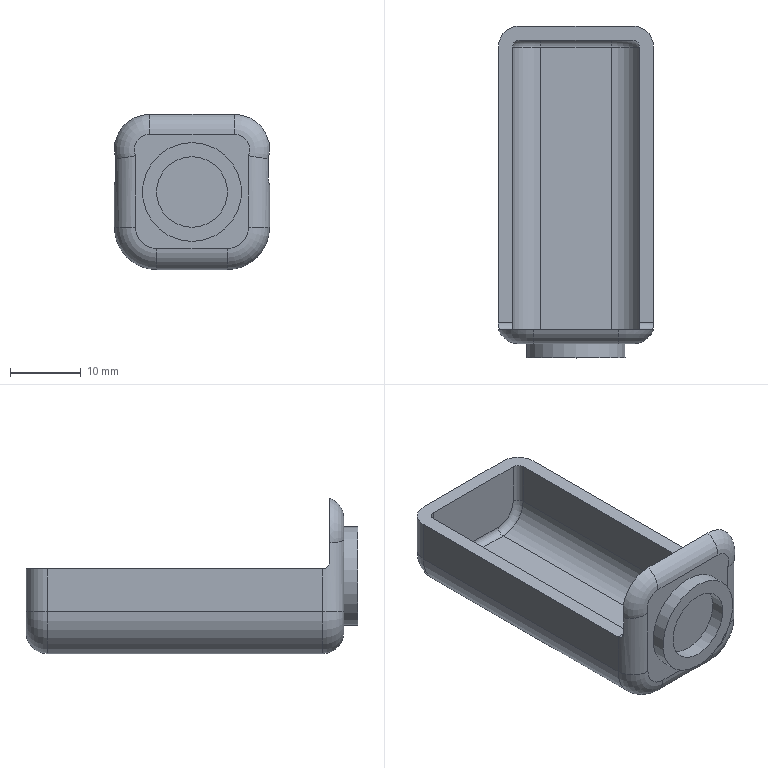Part | NX | features BLEND 5, DATUM_CSYS 4, SKETCH 3, EXTRUDE 2, SHELL 1, SWP104 1 | 1 solid | 39 faces | box 22 x 47 x 22 mm | volume 4457 mm3 | cylinder 18 | plane 13 | torus 8 | commonest cylinder face diameters 6 x7 2 x5 8 x2 12 x2 10 x1 14 x1
STEP:
#1=CARTESIAN_POINT('',(10.828,4.,2.));
#2=VERTEX_POINT('',#1);
#3=CARTESIAN_POINT('',(9.,4.,2.));
#4=VERTEX_POINT('',#3);
#5=CARTESIAN_POINT('',(-11.,4.,2.));
#6=DIRECTION('',(-1.,0.,0.));
#7=VECTOR('',#6,1000.);
#8=LINE('',#5,#7);
#9=EDGE_CURVE('',#2,#4,#8,.T.);
#10=ORIENTED_EDGE('',*,*,#9,.F.);
#11=CARTESIAN_POINT('',(11.,5.,1.));
#12=VERTEX_POINT('',#11);
#13=CARTESIAN_POINT('',(10.828,4.,2.));
#14=CARTESIAN_POINT('',(10.828,4.,1.468));
#15=CARTESIAN_POINT('',(11.,4.468,1.));
#16=CARTESIAN_POINT('',(11.,5.,1.));
#17=B_SPLINE_CURVE_WITH_KNOTS('',3,(#13,#14,#15,#16),.UNSPECIFIED.,.F.,.F.,(4,4),(0.,0.001574),.UNSPECIFIED.);
#18=EDGE_CURVE('',#2,#12,#17,.T.);
#19=ORIENTED_EDGE('',*,*,#18,.T.);
#20=CARTESIAN_POINT('',(9.,5.,1.));
#21=VERTEX_POINT('',#20);
#22=CARTESIAN_POINT('',(11.,5.,1.));
#23=DIRECTION('',(-1.,0.,0.));
#24=VECTOR('',#23,1000.);
#25=LINE('',#22,#24);
#26=EDGE_CURVE('',#21,#12,#25,.F.);
#27=ORIENTED_EDGE('',*,*,#26,.F.);
#28=CARTESIAN_POINT('',(9.,5.,2.));
#29=DIRECTION('',(-1.,0.,0.));
#30=DIRECTION('',(0.,0.,1.));
#31=AXIS2_PLACEMENT_3D('',#28,#29,#30);
#32=CIRCLE('',#31,1.);
#33=EDGE_CURVE('',#21,#4,#32,.T.);
#34=ORIENTED_EDGE('',*,*,#33,.T.);
#35=EDGE_LOOP('',(#10,#19,#27,#34));
#36=FACE_BOUND('',#35,.T.);
#37=CARTESIAN_POINT('',(-56.,5.,2.));
#38=DIRECTION('',(1.,0.,0.));
#39=DIRECTION('',(0.,0.,-1.));
#40=AXIS2_PLACEMENT_3D('',#37,#38,#39);
#41=CYLINDRICAL_SURFACE('',#40,1.);
#42=ADVANCED_FACE('',(#36),#41,.F.);
#43=CARTESIAN_POINT('',(-8.,47.,1.));
#44=VERTEX_POINT('',#43);
#45=CARTESIAN_POINT('',(8.,47.,1.));
#46=VERTEX_POINT('',#45);
#47=CARTESIAN_POINT('',(0.,47.,1.));
#48=DIRECTION('',(1.,0.,0.));
#49=VECTOR('',#48,1000.);
#50=LINE('',#47,#49);
#51=EDGE_CURVE('',#44,#46,#50,.T.);
#52=ORIENTED_EDGE('',*,*,#51,.T.);
#53=CARTESIAN_POINT('',(8.,47.,-5.));
#54=VERTEX_POINT('',#53);
#55=CARTESIAN_POINT('',(8.,47.,-5.));
#56=DIRECTION('',(0.,0.,-1.));
#57=VECTOR('',#56,1000.);
#58=LINE('',#55,#57);
#59=EDGE_CURVE('',#46,#54,#58,.T.);
#60=ORIENTED_EDGE('',*,*,#59,.T.);
#61=CARTESIAN_POINT('',(5.,47.,-8.));
#62=VERTEX_POINT('',#61);
#63=CARTESIAN_POINT('',(5.,47.,-5.));
#64=DIRECTION('',(0.,1.,0.));
#65=DIRECTION('',(0.,0.,1.));
#66=AXIS2_PLACEMENT_3D('',#63,#64,#65);
#67=CIRCLE('',#66,3.);
#68=EDGE_CURVE('',#54,#62,#67,.T.);
#69=ORIENTED_EDGE('',*,*,#68,.T.);
#70=CARTESIAN_POINT('',(-5.,47.,-8.));
#71=VERTEX_POINT('',#70);
#72=CARTESIAN_POINT('',(-5.,47.,-8.));
#73=DIRECTION('',(-1.,0.,0.));
#74=VECTOR('',#73,1000.);
#75=LINE('',#72,#74);
#76=EDGE_CURVE('',#62,#71,#75,.T.);
#77=ORIENTED_EDGE('',*,*,#76,.T.);
#78=CARTESIAN_POINT('',(-8.,47.,-5.));
#79=VERTEX_POINT('',#78);
#80=CARTESIAN_POINT('',(-5.,47.,-5.));
#81=DIRECTION('',(0.,1.,0.));
#82=DIRECTION('',(0.,0.,1.));
#83=AXIS2_PLACEMENT_3D('',#80,#81,#82);
#84=CIRCLE('',#83,3.);
#85=EDGE_CURVE('',#71,#79,#84,.T.);
#86=ORIENTED_EDGE('',*,*,#85,.T.);
#87=CARTESIAN_POINT('',(-8.,47.,1.));
#88=DIRECTION('',(0.,0.,1.));
#89=VECTOR('',#88,1000.);
#90=LINE('',#87,#89);
#91=EDGE_CURVE('',#79,#44,#90,.T.);
#92=ORIENTED_EDGE('',*,*,#91,.T.);
#93=EDGE_LOOP('',(#52,#60,#69,#77,#86,#92));
#94=FACE_BOUND('',#93,.T.);
#95=CARTESIAN_POINT('',(0.,47.,0.));
#96=DIRECTION('',(0.,1.,0.));
#97=DIRECTION('',(0.,0.,1.));
#98=AXIS2_PLACEMENT_3D('',#95,#96,#97);
#99=PLANE('',#98);
#100=ADVANCED_FACE('',(#94),#99,.T.);
#101=CARTESIAN_POINT('',(11.,44.,1.));
#102=VERTEX_POINT('',#101);
#103=CARTESIAN_POINT('',(11.,47.,1.));
#104=DIRECTION('',(0.,1.,0.));
#105=VECTOR('',#104,1000.);
#106=LINE('',#103,#105);
#107=EDGE_CURVE('',#12,#102,#106,.T.);
#108=ORIENTED_EDGE('',*,*,#107,.F.);
#109=CARTESIAN_POINT('',(11.,5.,-5.));
#110=VERTEX_POINT('',#109);
#111=CARTESIAN_POINT('',(11.,5.,11.));
#112=DIRECTION('',(0.,0.,-1.));
#113=VECTOR('',#112,1000.);
#114=LINE('',#111,#113);
#115=EDGE_CURVE('',#12,#110,#114,.T.);
#116=ORIENTED_EDGE('',*,*,#115,.T.);
#117=CARTESIAN_POINT('',(11.,44.,-5.));
#118=VERTEX_POINT('',#117);
#119=CARTESIAN_POINT('',(11.,47.,-5.));
#120=DIRECTION('',(0.,-1.,0.));
#121=VECTOR('',#120,1000.);
#122=LINE('',#119,#121);
#123=EDGE_CURVE('',#110,#118,#122,.F.);
#124=ORIENTED_EDGE('',*,*,#123,.T.);
#125=CARTESIAN_POINT('',(11.,44.,1.));
#126=DIRECTION('',(0.,0.,-1.));
#127=VECTOR('',#126,1000.);
#128=LINE('',#125,#127);
#129=EDGE_CURVE('',#118,#102,#128,.F.);
#130=ORIENTED_EDGE('',*,*,#129,.T.);
#131=EDGE_LOOP('',(#108,#116,#124,#130));
#132=FACE_BOUND('',#131,.T.);
#133=CARTESIAN_POINT('',(11.,47.,11.));
#134=DIRECTION('',(-1.,0.,0.));
#135=DIRECTION('',(0.,0.,1.));
#136=AXIS2_PLACEMENT_3D('',#133,#134,#135);
#137=PLANE('',#136);
#138=ADVANCED_FACE('',(#132),#137,.F.);
#139=CARTESIAN_POINT('',(-11.,44.,-5.));
#140=VERTEX_POINT('',#139);
#141=CARTESIAN_POINT('',(-11.,5.,-5.));
#142=VERTEX_POINT('',#141);
#143=CARTESIAN_POINT('',(-11.,47.,-5.));
#144=DIRECTION('',(0.,-1.,0.));
#145=VECTOR('',#144,1000.);
#146=LINE('',#143,#145);
#147=EDGE_CURVE('',#140,#142,#146,.T.);
#148=ORIENTED_EDGE('',*,*,#147,.T.);
#149=CARTESIAN_POINT('',(-11.,5.,1.));
#150=VERTEX_POINT('',#149);
#151=CARTESIAN_POINT('',(-11.,5.,-11.));
#152=DIRECTION('',(0.,0.,1.));
#153=VECTOR('',#152,1000.);
#154=LINE('',#151,#153);
#155=EDGE_CURVE('',#142,#150,#154,.T.);
#156=ORIENTED_EDGE('',*,*,#155,.T.);
#157=CARTESIAN_POINT('',(-11.,44.,1.));
#158=VERTEX_POINT('',#157);
#159=CARTESIAN_POINT('',(-11.,47.,1.));
#160=DIRECTION('',(0.,-1.,0.));
#161=VECTOR('',#160,1000.);
#162=LINE('',#159,#161);
#163=EDGE_CURVE('',#158,#150,#162,.T.);
#164=ORIENTED_EDGE('',*,*,#163,.F.);
#165=CARTESIAN_POINT('',(-11.,44.,-5.));
#166=DIRECTION('',(0.,0.,1.));
#167=VECTOR('',#166,1000.);
#168=LINE('',#165,#167);
#169=EDGE_CURVE('',#158,#140,#168,.F.);
#170=ORIENTED_EDGE('',*,*,#169,.T.);
#171=EDGE_LOOP('',(#148,#156,#164,#170));
#172=FACE_BOUND('',#171,.T.);
#173=CARTESIAN_POINT('',(-11.,47.,-11.));
#174=DIRECTION('',(1.,0.,0.));
#175=DIRECTION('',(0.,0.,-1.));
#176=AXIS2_PLACEMENT_3D('',#173,#174,#175);
#177=PLANE('',#176);
#178=ADVANCED_FACE('',(#172),#177,.F.);
#179=CARTESIAN_POINT('',(0.,0.,5.));
#180=VERTEX_POINT('',#179);
#181=CARTESIAN_POINT('',(0.,0.,0.));
#182=DIRECTION('',(0.,1.,0.));
#183=DIRECTION('',(0.,0.,1.));
#184=AXIS2_PLACEMENT_3D('',#181,#182,#183);
#185=CIRCLE('',#184,5.);
#186=EDGE_CURVE('',#180,#180,#185,.T.);
#187=ORIENTED_EDGE('',*,*,#186,.F.);
#188=EDGE_LOOP('',(#187));
#189=FACE_BOUND('',#188,.T.);
#190=CARTESIAN_POINT('',(0.,2.,5.));
#191=VERTEX_POINT('',#190);
#192=CARTESIAN_POINT('',(0.,2.,0.));
#193=DIRECTION('',(0.,1.,0.));
#194=DIRECTION('',(0.,0.,1.));
#195=AXIS2_PLACEMENT_3D('',#192,#193,#194);
#196=CIRCLE('',#195,5.);
#197=EDGE_CURVE('',#191,#191,#196,.T.);
#198=ORIENTED_EDGE('',*,*,#197,.T.);
#199=EDGE_LOOP('',(#198));
#200=FACE_BOUND('',#199,.T.);
#201=CARTESIAN_POINT('',(0.,0.,0.));
#202=DIRECTION('',(0.,1.,0.));
#203=DIRECTION('',(0.,0.,1.));
#204=AXIS2_PLACEMENT_3D('',#201,#202,#203);
#205=CYLINDRICAL_SURFACE('',#204,5.);
#206=ADVANCED_FACE('',(#189,#200),#205,.F.);
#207=CARTESIAN_POINT('',(0.,0.,7.));
#208=VERTEX_POINT('',#207);
#209=CARTESIAN_POINT('',(0.,0.,0.));
#210=DIRECTION('',(0.,1.,0.));
#211=DIRECTION('',(0.,0.,1.));
#212=AXIS2_PLACEMENT_3D('',#209,#210,#211);
#213=CIRCLE('',#212,7.);
#214=EDGE_CURVE('',#208,#208,#213,.T.);
#215=ORIENTED_EDGE('',*,*,#214,.F.);
#216=EDGE_LOOP('',(#215));
#217=FACE_BOUND('',#216,.T.);
#218=ORIENTED_EDGE('',*,*,#186,.T.);
#219=EDGE_LOOP('',(#218));
#220=FACE_BOUND('',#219,.T.);
#221=CARTESIAN_POINT('',(5.,0.,0.));
#222=DIRECTION('',(0.,1.,0.));
#223=DIRECTION('',(0.,0.,1.));
#224=AXIS2_PLACEMENT_3D('',#221,#222,#223);
#225=PLANE('',#224);
#226=ADVANCED_FACE('',(#217,#220),#225,.F.);
#227=CARTESIAN_POINT('',(0.,2.,7.));
#228=VERTEX_POINT('',#227);
#229=CARTESIAN_POINT('',(0.,2.,0.));
#230=DIRECTION('',(0.,1.,0.));
#231=DIRECTION('',(0.,0.,1.));
#232=AXIS2_PLACEMENT_3D('',#229,#230,#231);
#233=CIRCLE('',#232,7.);
#234=EDGE_CURVE('',#228,#228,#233,.T.);
#235=ORIENTED_EDGE('',*,*,#234,.F.);
#236=EDGE_LOOP('',(#235));
#237=FACE_BOUND('',#236,.T.);
#238=ORIENTED_EDGE('',*,*,#214,.T.);
#239=EDGE_LOOP('',(#238));
#240=FACE_BOUND('',#239,.T.);
#241=CARTESIAN_POINT('',(0.,0.,0.));
#242=DIRECTION('',(0.,1.,0.));
#243=DIRECTION('',(0.,0.,1.));
#244=AXIS2_PLACEMENT_3D('',#241,#242,#243);
#245=CYLINDRICAL_SURFACE('',#244,7.);
#246=ADVANCED_FACE('',(#237,#240),#245,.T.);
#247=CARTESIAN_POINT('',(-8.,2.,-5.));
#248=VERTEX_POINT('',#247);
#249=CARTESIAN_POINT('',(-5.,2.,-8.));
#250=VERTEX_POINT('',#249);
#251=CARTESIAN_POINT('',(-5.,2.,-5.));
#252=DIRECTION('',(0.,1.,0.));
#253=DIRECTION('',(0.,0.,1.));
#254=AXIS2_PLACEMENT_3D('',#251,#252,#253);
#255=CIRCLE('',#254,3.);
#256=EDGE_CURVE('',#248,#250,#255,.F.);
#257=ORIENTED_EDGE('',*,*,#256,.T.);
#258=CARTESIAN_POINT('',(5.,2.,-8.));
#259=VERTEX_POINT('',#258);
#260=CARTESIAN_POINT('',(0.,2.,-8.));
#261=DIRECTION('',(-1.,0.,0.));
#262=VECTOR('',#261,1000.);
#263=LINE('',#260,#262);
#264=EDGE_CURVE('',#250,#259,#263,.F.);
#265=ORIENTED_EDGE('',*,*,#264,.T.);
#266=CARTESIAN_POINT('',(8.,2.,-5.));
#267=VERTEX_POINT('',#266);
#268=CARTESIAN_POINT('',(5.,2.,-5.));
#269=DIRECTION('',(0.,1.,0.));
#270=DIRECTION('',(0.,0.,1.));
#271=AXIS2_PLACEMENT_3D('',#268,#269,#270);
#272=CIRCLE('',#271,3.);
#273=EDGE_CURVE('',#259,#267,#272,.F.);
#274=ORIENTED_EDGE('',*,*,#273,.T.);
#275=CARTESIAN_POINT('',(8.,2.,5.154));
#276=VERTEX_POINT('',#275);
#277=CARTESIAN_POINT('',(8.,2.,0.));
#278=DIRECTION('',(0.,0.,-1.));
#279=VECTOR('',#278,1000.);
#280=LINE('',#277,#279);
#281=EDGE_CURVE('',#267,#276,#280,.F.);
#282=ORIENTED_EDGE('',*,*,#281,.T.);
#283=CARTESIAN_POINT('',(6.,2.,8.172));
#284=VERTEX_POINT('',#283);
#285=CARTESIAN_POINT('',(6.,2.,6.));
#286=DIRECTION('',(0.,1.,0.));
#287=DIRECTION('',(0.,0.,1.));
#288=AXIS2_PLACEMENT_3D('',#285,#286,#287);
#289=CIRCLE('',#288,2.172);
#290=EDGE_CURVE('',#276,#284,#289,.F.);
#291=ORIENTED_EDGE('',*,*,#290,.T.);
#292=CARTESIAN_POINT('',(-6.,2.,8.172));
#293=VERTEX_POINT('',#292);
#294=CARTESIAN_POINT('',(0.,2.,8.172));
#295=DIRECTION('',(1.,0.,0.));
#296=VECTOR('',#295,1000.);
#297=LINE('',#294,#296);
#298=EDGE_CURVE('',#284,#293,#297,.F.);
#299=ORIENTED_EDGE('',*,*,#298,.T.);
#300=CARTESIAN_POINT('',(-8.,2.,5.154));
#301=VERTEX_POINT('',#300);
#302=CARTESIAN_POINT('',(-6.,2.,6.));
#303=DIRECTION('',(0.,1.,0.));
#304=DIRECTION('',(0.,0.,1.));
#305=AXIS2_PLACEMENT_3D('',#302,#303,#304);
#306=CIRCLE('',#305,2.172);
#307=EDGE_CURVE('',#293,#301,#306,.F.);
#308=ORIENTED_EDGE('',*,*,#307,.T.);
#309=CARTESIAN_POINT('',(-8.,2.,0.));
#310=DIRECTION('',(0.,0.,1.));
#311=VECTOR('',#310,1000.);
#312=LINE('',#309,#311);
#313=EDGE_CURVE('',#301,#248,#312,.F.);
#314=ORIENTED_EDGE('',*,*,#313,.T.);
#315=EDGE_LOOP('',(#257,#265,#274,#282,#291,#299,#308,#314));
#316=FACE_BOUND('',#315,.T.);
#317=ORIENTED_EDGE('',*,*,#234,.T.);
#318=EDGE_LOOP('',(#317));
#319=FACE_BOUND('',#318,.T.);
#320=CARTESIAN_POINT('',(0.,2.,0.));
#321=DIRECTION('',(0.,1.,0.));
#322=DIRECTION('',(0.,0.,1.));
#323=AXIS2_PLACEMENT_3D('',#320,#321,#322);
#324=PLANE('',#323);
#325=ADVANCED_FACE('',(#316,#319),#324,.F.);
#326=CARTESIAN_POINT('',(5.,44.,-11.));
#327=VERTEX_POINT('',#326);
#328=CARTESIAN_POINT('',(5.,5.,-11.));
#329=VERTEX_POINT('',#328);
#330=CARTESIAN_POINT('',(5.,47.,-11.));
#331=DIRECTION('',(0.,-1.,0.));
#332=VECTOR('',#331,1000.);
#333=LINE('',#330,#332);
#334=EDGE_CURVE('',#327,#329,#333,.T.);
#335=ORIENTED_EDGE('',*,*,#334,.T.);
#336=CARTESIAN_POINT('',(-5.,5.,-11.));
#337=VERTEX_POINT('',#336);
#338=CARTESIAN_POINT('',(11.,5.,-11.));
#339=DIRECTION('',(-1.,0.,0.));
#340=VECTOR('',#339,1000.);
#341=LINE('',#338,#340);
#342=EDGE_CURVE('',#329,#337,#341,.T.);
#343=ORIENTED_EDGE('',*,*,#342,.T.);
#344=CARTESIAN_POINT('',(-5.,44.,-11.));
#345=VERTEX_POINT('',#344);
#346=CARTESIAN_POINT('',(-5.,47.,-11.));
#347=DIRECTION('',(0.,-1.,0.));
#348=VECTOR('',#347,1000.);
#349=LINE('',#346,#348);
#350=EDGE_CURVE('',#337,#345,#349,.F.);
#351=ORIENTED_EDGE('',*,*,#350,.T.);
#352=CARTESIAN_POINT('',(5.,44.,-11.));
#353=DIRECTION('',(-1.,0.,0.));
#354=VECTOR('',#353,1000.);
#355=LINE('',#352,#354);
#356=EDGE_CURVE('',#345,#327,#355,.F.);
#357=ORIENTED_EDGE('',*,*,#356,.T.);
#358=EDGE_LOOP('',(#335,#343,#351,#357));
#359=FACE_BOUND('',#358,.T.);
#360=CARTESIAN_POINT('',(11.,47.,-11.));
#361=DIRECTION('',(0.,0.,1.));
#362=DIRECTION('',(1.,0.,0.));
#363=AXIS2_PLACEMENT_3D('',#360,#361,#362);
#364=PLANE('',#363);
#365=ADVANCED_FACE('',(#359),#364,.F.);
#366=ORIENTED_EDGE('',*,*,#197,.F.);
#367=EDGE_LOOP('',(#366));
#368=FACE_BOUND('',#367,.T.);
#369=CARTESIAN_POINT('',(0.,2.,0.));
#370=DIRECTION('',(0.,1.,0.));
#371=DIRECTION('',(0.,0.,1.));
#372=AXIS2_PLACEMENT_3D('',#369,#370,#371);
#373=PLANE('',#372);
#374=ADVANCED_FACE('',(#368),#373,.F.);
#375=CARTESIAN_POINT('',(-6.,4.,11.));
#376=VERTEX_POINT('',#375);
#377=CARTESIAN_POINT('',(6.,4.,11.));
#378=VERTEX_POINT('',#377);
#379=CARTESIAN_POINT('',(-56.,4.,11.));
#380=DIRECTION('',(1.,0.,0.));
#381=VECTOR('',#380,1000.);
#382=LINE('',#379,#381);
#383=EDGE_CURVE('',#376,#378,#382,.T.);
#384=ORIENTED_EDGE('',*,*,#383,.T.);
#385=CARTESIAN_POINT('',(10.828,4.,4.701));
#386=VERTEX_POINT('',#385);
#387=CARTESIAN_POINT('',(6.,4.,6.));
#388=DIRECTION('',(0.,1.,0.));
#389=DIRECTION('',(0.,0.,1.));
#390=AXIS2_PLACEMENT_3D('',#387,#388,#389);
#391=CIRCLE('',#390,5.);
#392=EDGE_CURVE('',#378,#386,#391,.T.);
#393=ORIENTED_EDGE('',*,*,#392,.T.);
#394=CARTESIAN_POINT('',(10.828,4.,4.701));
#395=DIRECTION('',(0.,0.,-1.));
#396=VECTOR('',#395,1000.);
#397=LINE('',#394,#396);
#398=EDGE_CURVE('',#386,#2,#397,.T.);
#399=ORIENTED_EDGE('',*,*,#398,.T.);
#400=ORIENTED_EDGE('',*,*,#9,.T.);
#401=CARTESIAN_POINT('',(9.,4.,-5.));
#402=VERTEX_POINT('',#401);
#403=CARTESIAN_POINT('',(9.,4.,11.));
#404=DIRECTION('',(0.,0.,-1.));
#405=VECTOR('',#404,1000.);
#406=LINE('',#403,#405);
#407=EDGE_CURVE('',#4,#402,#406,.T.);
#408=ORIENTED_EDGE('',*,*,#407,.T.);
#409=CARTESIAN_POINT('',(5.,4.,-9.));
#410=VERTEX_POINT('',#409);
#411=CARTESIAN_POINT('',(5.,4.,-5.));
#412=DIRECTION('',(0.,1.,0.));
#413=DIRECTION('',(0.,0.,1.));
#414=AXIS2_PLACEMENT_3D('',#411,#412,#413);
#415=CIRCLE('',#414,4.);
#416=EDGE_CURVE('',#410,#402,#415,.F.);
#417=ORIENTED_EDGE('',*,*,#416,.F.);
#418=CARTESIAN_POINT('',(-5.,4.,-9.));
#419=VERTEX_POINT('',#418);
#420=CARTESIAN_POINT('',(11.,4.,-9.));
#421=DIRECTION('',(-1.,0.,0.));
#422=VECTOR('',#421,1000.);
#423=LINE('',#420,#422);
#424=EDGE_CURVE('',#410,#419,#423,.T.);
#425=ORIENTED_EDGE('',*,*,#424,.T.);
#426=CARTESIAN_POINT('',(-9.,4.,-5.));
#427=VERTEX_POINT('',#426);
#428=CARTESIAN_POINT('',(-5.,4.,-5.));
#429=DIRECTION('',(0.,1.,0.));
#430=DIRECTION('',(0.,0.,1.));
#431=AXIS2_PLACEMENT_3D('',#428,#429,#430);
#432=CIRCLE('',#431,4.);
#433=EDGE_CURVE('',#427,#419,#432,.F.);
#434=ORIENTED_EDGE('',*,*,#433,.F.);
#435=CARTESIAN_POINT('',(-9.,4.,2.));
#436=VERTEX_POINT('',#435);
#437=CARTESIAN_POINT('',(-9.,4.,-11.));
#438=DIRECTION('',(0.,0.,1.));
#439=VECTOR('',#438,1000.);
#440=LINE('',#437,#439);
#441=EDGE_CURVE('',#427,#436,#440,.T.);
#442=ORIENTED_EDGE('',*,*,#441,.T.);
#443=CARTESIAN_POINT('',(-10.828,4.,2.));
#444=VERTEX_POINT('',#443);
#445=CARTESIAN_POINT('',(-11.,4.,2.));
#446=DIRECTION('',(-1.,0.,0.));
#447=VECTOR('',#446,1000.);
#448=LINE('',#445,#447);
#449=EDGE_CURVE('',#436,#444,#448,.T.);
#450=ORIENTED_EDGE('',*,*,#449,.T.);
#451=CARTESIAN_POINT('',(-10.828,4.,4.701));
#452=VERTEX_POINT('',#451);
#453=CARTESIAN_POINT('',(-10.828,4.,2.));
#454=DIRECTION('',(0.,0.,1.));
#455=VECTOR('',#454,1000.);
#456=LINE('',#453,#455);
#457=EDGE_CURVE('',#444,#452,#456,.T.);
#458=ORIENTED_EDGE('',*,*,#457,.T.);
#459=CARTESIAN_POINT('',(-6.,4.,6.));
#460=DIRECTION('',(0.,1.,0.));
#461=DIRECTION('',(0.,0.,1.));
#462=AXIS2_PLACEMENT_3D('',#459,#460,#461);
#463=CIRCLE('',#462,5.);
#464=EDGE_CURVE('',#452,#376,#463,.T.);
#465=ORIENTED_EDGE('',*,*,#464,.T.);
#466=EDGE_LOOP('',(#384,#393,#399,#400,#408,#417,#425,#434,#442,#450,#458,#465));
#467=FACE_BOUND('',#466,.T.);
#468=CARTESIAN_POINT('',(-56.,4.,1.));
#469=DIRECTION('',(0.,1.,0.));
#470=DIRECTION('',(0.,0.,1.));
#471=AXIS2_PLACEMENT_3D('',#468,#469,#470);
#472=PLANE('',#471);
#473=ADVANCED_FACE('',(#467),#472,.T.);
#474=CARTESIAN_POINT('',(9.,44.,1.));
#475=VERTEX_POINT('',#474);
#476=CARTESIAN_POINT('',(9.,47.,1.));
#477=DIRECTION('',(0.,1.,0.));
#478=VECTOR('',#477,1000.);
#479=LINE('',#476,#478);
#480=EDGE_CURVE('',#21,#475,#479,.T.);
#481=ORIENTED_EDGE('',*,*,#480,.F.);
#482=ORIENTED_EDGE('',*,*,#26,.T.);
#483=ORIENTED_EDGE('',*,*,#107,.T.);
#484=CARTESIAN_POINT('',(8.,44.,1.));
#485=DIRECTION('',(0.,0.,1.));
#486=DIRECTION('',(1.,0.,0.));
#487=AXIS2_PLACEMENT_3D('',#484,#485,#486);
#488=CIRCLE('',#487,3.);
#489=EDGE_CURVE('',#102,#46,#488,.T.);
#490=ORIENTED_EDGE('',*,*,#489,.T.);
#491=ORIENTED_EDGE('',*,*,#51,.F.);
#492=CARTESIAN_POINT('',(-8.,44.,1.));
#493=DIRECTION('',(0.,0.,1.));
#494=DIRECTION('',(1.,0.,0.));
#495=AXIS2_PLACEMENT_3D('',#492,#493,#494);
#496=CIRCLE('',#495,3.);
#497=EDGE_CURVE('',#44,#158,#496,.T.);
#498=ORIENTED_EDGE('',*,*,#497,.T.);
#499=ORIENTED_EDGE('',*,*,#163,.T.);
#500=CARTESIAN_POINT('',(-9.,5.,1.));
#501=VERTEX_POINT('',#500);
#502=CARTESIAN_POINT('',(11.,5.,1.));
#503=DIRECTION('',(-1.,0.,0.));
#504=VECTOR('',#503,1000.);
#505=LINE('',#502,#504);
#506=EDGE_CURVE('',#150,#501,#505,.F.);
#507=ORIENTED_EDGE('',*,*,#506,.T.);
#508=CARTESIAN_POINT('',(-9.,44.,1.));
#509=VERTEX_POINT('',#508);
#510=CARTESIAN_POINT('',(-9.,47.,1.));
#511=DIRECTION('',(0.,-1.,0.));
#512=VECTOR('',#511,1000.);
#513=LINE('',#510,#512);
#514=EDGE_CURVE('',#509,#501,#513,.T.);
#515=ORIENTED_EDGE('',*,*,#514,.F.);
#516=CARTESIAN_POINT('',(-8.,45.,1.));
#517=VERTEX_POINT('',#516);
#518=CARTESIAN_POINT('',(-8.,44.,1.));
#519=DIRECTION('',(0.,0.,1.));
#520=DIRECTION('',(1.,0.,0.));
#521=AXIS2_PLACEMENT_3D('',#518,#519,#520);
#522=CIRCLE('',#521,1.);
#523=EDGE_CURVE('',#517,#509,#522,.T.);
#524=ORIENTED_EDGE('',*,*,#523,.F.);
#525=CARTESIAN_POINT('',(8.,45.,1.));
#526=VERTEX_POINT('',#525);
#527=CARTESIAN_POINT('',(0.,45.,1.));
#528=DIRECTION('',(1.,0.,0.));
#529=VECTOR('',#528,1000.);
#530=LINE('',#527,#529);
#531=EDGE_CURVE('',#517,#526,#530,.T.);
#532=ORIENTED_EDGE('',*,*,#531,.T.);
#533=CARTESIAN_POINT('',(8.,44.,1.));
#534=DIRECTION('',(0.,0.,1.));
#535=DIRECTION('',(1.,0.,0.));
#536=AXIS2_PLACEMENT_3D('',#533,#534,#535);
#537=CIRCLE('',#536,1.);
#538=EDGE_CURVE('',#475,#526,#537,.T.);
#539=ORIENTED_EDGE('',*,*,#538,.F.);
#540=EDGE_LOOP('',(#481,#482,#483,#490,#491,#498,#499,#507,#515,#524,#532,#539));
#541=FACE_BOUND('',#540,.T.);
#542=CARTESIAN_POINT('',(-56.,54.5,1.));
#543=DIRECTION('',(0.,0.,1.));
#544=DIRECTION('',(1.,0.,0.));
#545=AXIS2_PLACEMENT_3D('',#542,#543,#544);
#546=PLANE('',#545);
#547=ADVANCED_FACE('',(#541),#546,.T.);
#548=ORIENTED_EDGE('',*,*,#350,.F.);
#549=CARTESIAN_POINT('',(-5.,5.,-5.));
#550=DIRECTION('',(0.,1.,0.));
#551=DIRECTION('',(0.,0.,1.));
#552=AXIS2_PLACEMENT_3D('',#549,#550,#551);
#553=CIRCLE('',#552,6.);
#554=EDGE_CURVE('',#337,#142,#553,.T.);
#555=ORIENTED_EDGE('',*,*,#554,.T.);
#556=ORIENTED_EDGE('',*,*,#147,.F.);
#557=CARTESIAN_POINT('',(-5.,44.,-5.));
#558=DIRECTION('',(0.,1.,0.));
#559=DIRECTION('',(0.,0.,1.));
#560=AXIS2_PLACEMENT_3D('',#557,#558,#559);
#561=CIRCLE('',#560,6.);
#562=EDGE_CURVE('',#140,#345,#561,.F.);
#563=ORIENTED_EDGE('',*,*,#562,.T.);
#564=EDGE_LOOP('',(#548,#555,#556,#563));
#565=FACE_BOUND('',#564,.T.);
#566=CARTESIAN_POINT('',(-5.,47.,-5.));
#567=DIRECTION('',(0.,-1.,0.));
#568=DIRECTION('',(0.,0.,-1.));
#569=AXIS2_PLACEMENT_3D('',#566,#567,#568);
#570=CYLINDRICAL_SURFACE('',#569,6.);
#571=ADVANCED_FACE('',(#565),#570,.T.);
#572=ORIENTED_EDGE('',*,*,#123,.F.);
#573=CARTESIAN_POINT('',(5.,5.,-5.));
#574=DIRECTION('',(0.,1.,0.));
#575=DIRECTION('',(0.,0.,1.));
#576=AXIS2_PLACEMENT_3D('',#573,#574,#575);
#577=CIRCLE('',#576,6.);
#578=EDGE_CURVE('',#110,#329,#577,.T.);
#579=ORIENTED_EDGE('',*,*,#578,.T.);
#580=ORIENTED_EDGE('',*,*,#334,.F.);
#581=CARTESIAN_POINT('',(5.,44.,-5.));
#582=DIRECTION('',(0.,1.,0.));
#583=DIRECTION('',(0.,0.,1.));
#584=AXIS2_PLACEMENT_3D('',#581,#582,#583);
#585=CIRCLE('',#584,6.);
#586=EDGE_CURVE('',#327,#118,#585,.F.);
#587=ORIENTED_EDGE('',*,*,#586,.T.);
#588=EDGE_LOOP('',(#572,#579,#580,#587));
#589=FACE_BOUND('',#588,.T.);
#590=CARTESIAN_POINT('',(5.,47.,-5.));
#591=DIRECTION('',(0.,-1.,0.));
#592=DIRECTION('',(0.,0.,-1.));
#593=AXIS2_PLACEMENT_3D('',#590,#591,#592);
#594=CYLINDRICAL_SURFACE('',#593,6.);
#595=ADVANCED_FACE('',(#589),#594,.T.);
#596=ORIENTED_EDGE('',*,*,#506,.F.);
#597=CARTESIAN_POINT('',(-11.,5.,1.));
#598=CARTESIAN_POINT('',(-11.,4.468,1.));
#599=CARTESIAN_POINT('',(-10.828,4.,1.468));
#600=CARTESIAN_POINT('',(-10.828,4.,2.));
#601=B_SPLINE_CURVE_WITH_KNOTS('',3,(#597,#598,#599,#600),.UNSPECIFIED.,.F.,.F.,(4,4),(0.,0.001574),.UNSPECIFIED.);
#602=EDGE_CURVE('',#150,#444,#601,.T.);
#603=ORIENTED_EDGE('',*,*,#602,.T.);
#604=ORIENTED_EDGE('',*,*,#449,.F.);
#605=CARTESIAN_POINT('',(-9.,5.,2.));
#606=DIRECTION('',(1.,0.,0.));
#607=DIRECTION('',(0.,0.,-1.));
#608=AXIS2_PLACEMENT_3D('',#605,#606,#607);
#609=CIRCLE('',#608,1.);
#610=EDGE_CURVE('',#436,#501,#609,.T.);
#611=ORIENTED_EDGE('',*,*,#610,.T.);
#612=EDGE_LOOP('',(#596,#603,#604,#611));
#613=FACE_BOUND('',#612,.T.);
#614=CARTESIAN_POINT('',(-56.,5.,2.));
#615=DIRECTION('',(1.,0.,0.));
#616=DIRECTION('',(0.,0.,-1.));
#617=AXIS2_PLACEMENT_3D('',#614,#615,#616);
#618=CYLINDRICAL_SURFACE('',#617,1.);
#619=ADVANCED_FACE('',(#613),#618,.F.);
#620=ORIENTED_EDGE('',*,*,#497,.F.);
#621=ORIENTED_EDGE('',*,*,#91,.F.);
#622=CARTESIAN_POINT('',(-8.,44.,-5.));
#623=DIRECTION('',(0.,0.,-1.));
#624=DIRECTION('',(-1.,0.,0.));
#625=AXIS2_PLACEMENT_3D('',#622,#623,#624);
#626=CIRCLE('',#625,3.);
#627=EDGE_CURVE('',#140,#79,#626,.T.);
#628=ORIENTED_EDGE('',*,*,#627,.F.);
#629=ORIENTED_EDGE('',*,*,#169,.F.);
#630=EDGE_LOOP('',(#620,#621,#628,#629));
#631=FACE_BOUND('',#630,.T.);
#632=CARTESIAN_POINT('',(-8.,44.,0.));
#633=DIRECTION('',(0.,0.,-1.));
#634=DIRECTION('',(-1.,0.,0.));
#635=AXIS2_PLACEMENT_3D('',#632,#633,#634);
#636=CYLINDRICAL_SURFACE('',#635,3.);
#637=ADVANCED_FACE('',(#631),#636,.T.);
#638=ORIENTED_EDGE('',*,*,#627,.T.);
#639=ORIENTED_EDGE('',*,*,#85,.F.);
#640=CARTESIAN_POINT('',(-5.,44.,-8.));
#641=DIRECTION('',(1.,0.,0.));
#642=DIRECTION('',(0.,0.,-1.));
#643=AXIS2_PLACEMENT_3D('',#640,#641,#642);
#644=CIRCLE('',#643,3.);
#645=EDGE_CURVE('',#345,#71,#644,.T.);
#646=ORIENTED_EDGE('',*,*,#645,.F.);
#647=ORIENTED_EDGE('',*,*,#562,.F.);
#648=EDGE_LOOP('',(#638,#639,#646,#647));
#649=FACE_BOUND('',#648,.T.);
#650=CARTESIAN_POINT('',(-5.,44.,-5.));
#651=DIRECTION('',(0.,1.,0.));
#652=DIRECTION('',(0.,0.,1.));
#653=AXIS2_PLACEMENT_3D('',#650,#651,#652);
#654=TOROIDAL_SURFACE('',#653,3.,3.);
#655=ADVANCED_FACE('',(#649),#654,.T.);
#656=ORIENTED_EDGE('',*,*,#645,.T.);
#657=ORIENTED_EDGE('',*,*,#76,.F.);
#658=CARTESIAN_POINT('',(5.,44.,-8.));
#659=DIRECTION('',(1.,0.,0.));
#660=DIRECTION('',(0.,0.,-1.));
#661=AXIS2_PLACEMENT_3D('',#658,#659,#660);
#662=CIRCLE('',#661,3.);
#663=EDGE_CURVE('',#327,#62,#662,.T.);
#664=ORIENTED_EDGE('',*,*,#663,.F.);
#665=ORIENTED_EDGE('',*,*,#356,.F.);
#666=EDGE_LOOP('',(#656,#657,#664,#665));
#667=FACE_BOUND('',#666,.T.);
#668=CARTESIAN_POINT('',(0.,44.,-8.));
#669=DIRECTION('',(1.,0.,0.));
#670=DIRECTION('',(0.,0.,-1.));
#671=AXIS2_PLACEMENT_3D('',#668,#669,#670);
#672=CYLINDRICAL_SURFACE('',#671,3.);
#673=ADVANCED_FACE('',(#667),#672,.T.);
#674=ORIENTED_EDGE('',*,*,#663,.T.);
#675=ORIENTED_EDGE('',*,*,#68,.F.);
#676=CARTESIAN_POINT('',(8.,44.,-5.));
#677=DIRECTION('',(0.,0.,1.));
#678=DIRECTION('',(1.,0.,0.));
#679=AXIS2_PLACEMENT_3D('',#676,#677,#678);
#680=CIRCLE('',#679,3.);
#681=EDGE_CURVE('',#118,#54,#680,.T.);
#682=ORIENTED_EDGE('',*,*,#681,.F.);
#683=ORIENTED_EDGE('',*,*,#586,.F.);
#684=EDGE_LOOP('',(#674,#675,#682,#683));
#685=FACE_BOUND('',#684,.T.);
#686=CARTESIAN_POINT('',(5.,44.,-5.));
#687=DIRECTION('',(0.,1.,0.));
#688=DIRECTION('',(0.,0.,1.));
#689=AXIS2_PLACEMENT_3D('',#686,#687,#688);
#690=TOROIDAL_SURFACE('',#689,3.,3.);
#691=ADVANCED_FACE('',(#685),#690,.T.);
#692=ORIENTED_EDGE('',*,*,#489,.F.);
#693=ORIENTED_EDGE('',*,*,#129,.F.);
#694=ORIENTED_EDGE('',*,*,#681,.T.);
#695=ORIENTED_EDGE('',*,*,#59,.F.);
#696=EDGE_LOOP('',(#692,#693,#694,#695));
#697=FACE_BOUND('',#696,.T.);
#698=CARTESIAN_POINT('',(8.,44.,0.));
#699=DIRECTION('',(0.,0.,1.));
#700=DIRECTION('',(1.,0.,0.));
#701=AXIS2_PLACEMENT_3D('',#698,#699,#700);
#702=CYLINDRICAL_SURFACE('',#701,3.);
#703=ADVANCED_FACE('',(#697),#702,.T.);
#704=ORIENTED_EDGE('',*,*,#531,.F.);
#705=CARTESIAN_POINT('',(-8.,45.,-5.));
#706=VERTEX_POINT('',#705);
#707=CARTESIAN_POINT('',(-8.,45.,0.));
#708=DIRECTION('',(0.,0.,1.));
#709=VECTOR('',#708,1000.);
#710=LINE('',#707,#709);
#711=EDGE_CURVE('',#706,#517,#710,.T.);
#712=ORIENTED_EDGE('',*,*,#711,.F.);
#713=CARTESIAN_POINT('',(-5.,45.,-8.));
#714=VERTEX_POINT('',#713);
#715=CARTESIAN_POINT('',(-5.,45.,-5.));
#716=DIRECTION('',(0.,1.,0.));
#717=DIRECTION('',(0.,0.,1.));
#718=AXIS2_PLACEMENT_3D('',#715,#716,#717);
#719=CIRCLE('',#718,3.);
#720=EDGE_CURVE('',#714,#706,#719,.T.);
#721=ORIENTED_EDGE('',*,*,#720,.F.);
#722=CARTESIAN_POINT('',(5.,45.,-8.));
#723=VERTEX_POINT('',#722);
#724=CARTESIAN_POINT('',(0.,45.,-8.));
#725=DIRECTION('',(1.,0.,0.));
#726=VECTOR('',#725,1000.);
#727=LINE('',#724,#726);
#728=EDGE_CURVE('',#723,#714,#727,.F.);
#729=ORIENTED_EDGE('',*,*,#728,.F.);
#730=CARTESIAN_POINT('',(8.,45.,-5.));
#731=VERTEX_POINT('',#730);
#732=CARTESIAN_POINT('',(5.,45.,-5.));
#733=DIRECTION('',(0.,1.,0.));
#734=DIRECTION('',(0.,0.,1.));
#735=AXIS2_PLACEMENT_3D('',#732,#733,#734);
#736=CIRCLE('',#735,3.);
#737=EDGE_CURVE('',#731,#723,#736,.T.);
#738=ORIENTED_EDGE('',*,*,#737,.F.);
#739=CARTESIAN_POINT('',(8.,45.,0.));
#740=DIRECTION('',(0.,0.,1.));
#741=VECTOR('',#740,1000.);
#742=LINE('',#739,#741);
#743=EDGE_CURVE('',#526,#731,#742,.F.);
#744=ORIENTED_EDGE('',*,*,#743,.F.);
#745=EDGE_LOOP('',(#704,#712,#721,#729,#738,#744));
#746=FACE_BOUND('',#745,.T.);
#747=CARTESIAN_POINT('',(0.,45.,0.));
#748=DIRECTION('',(0.,1.,0.));
#749=DIRECTION('',(0.,0.,1.));
#750=AXIS2_PLACEMENT_3D('',#747,#748,#749);
#751=PLANE('',#750);
#752=ADVANCED_FACE('',(#746),#751,.F.);
#753=CARTESIAN_POINT('',(9.,44.,-5.));
#754=VERTEX_POINT('',#753);
#755=CARTESIAN_POINT('',(9.,47.,-5.));
#756=DIRECTION('',(0.,1.,0.));
#757=VECTOR('',#756,1000.);
#758=LINE('',#755,#757);
#759=EDGE_CURVE('',#402,#754,#758,.T.);
#760=ORIENTED_EDGE('',*,*,#759,.F.);
#761=ORIENTED_EDGE('',*,*,#407,.F.);
#762=ORIENTED_EDGE('',*,*,#33,.F.);
#763=ORIENTED_EDGE('',*,*,#480,.T.);
#764=CARTESIAN_POINT('',(9.,44.,11.));
#765=DIRECTION('',(0.,0.,1.));
#766=VECTOR('',#765,1000.);
#767=LINE('',#764,#766);
#768=EDGE_CURVE('',#754,#475,#767,.T.);
#769=ORIENTED_EDGE('',*,*,#768,.F.);
#770=EDGE_LOOP('',(#760,#761,#762,#763,#769));
#771=FACE_BOUND('',#770,.T.);
#772=CARTESIAN_POINT('',(9.,47.,11.));
#773=DIRECTION('',(-1.,0.,0.));
#774=DIRECTION('',(0.,0.,1.));
#775=AXIS2_PLACEMENT_3D('',#772,#773,#774);
#776=PLANE('',#775);
#777=ADVANCED_FACE('',(#771),#776,.T.);
#778=ORIENTED_EDGE('',*,*,#514,.T.);
#779=ORIENTED_EDGE('',*,*,#610,.F.);
#780=ORIENTED_EDGE('',*,*,#441,.F.);
#781=CARTESIAN_POINT('',(-9.,44.,-5.));
#782=VERTEX_POINT('',#781);
#783=CARTESIAN_POINT('',(-9.,47.,-5.));
#784=DIRECTION('',(0.,1.,0.));
#785=VECTOR('',#784,1000.);
#786=LINE('',#783,#785);
#787=EDGE_CURVE('',#782,#427,#786,.F.);
#788=ORIENTED_EDGE('',*,*,#787,.F.);
#789=CARTESIAN_POINT('',(-9.,44.,-11.));
#790=DIRECTION('',(0.,0.,-1.));
#791=VECTOR('',#790,1000.);
#792=LINE('',#789,#791);
#793=EDGE_CURVE('',#509,#782,#792,.T.);
#794=ORIENTED_EDGE('',*,*,#793,.F.);
#795=EDGE_LOOP('',(#778,#779,#780,#788,#794));
#796=FACE_BOUND('',#795,.T.);
#797=CARTESIAN_POINT('',(-9.,47.,-11.));
#798=DIRECTION('',(1.,0.,0.));
#799=DIRECTION('',(0.,0.,-1.));
#800=AXIS2_PLACEMENT_3D('',#797,#798,#799);
#801=PLANE('',#800);
#802=ADVANCED_FACE('',(#796),#801,.T.);
#803=CARTESIAN_POINT('',(-5.,44.,-9.));
#804=VERTEX_POINT('',#803);
#805=CARTESIAN_POINT('',(-5.,47.,-9.));
#806=DIRECTION('',(0.,1.,0.));
#807=VECTOR('',#806,1000.);
#808=LINE('',#805,#807);
#809=EDGE_CURVE('',#419,#804,#808,.T.);
#810=ORIENTED_EDGE('',*,*,#809,.F.);
#811=ORIENTED_EDGE('',*,*,#424,.F.);
#812=CARTESIAN_POINT('',(5.,44.,-9.));
#813=VERTEX_POINT('',#812);
#814=CARTESIAN_POINT('',(5.,47.,-9.));
#815=DIRECTION('',(0.,1.,0.));
#816=VECTOR('',#815,1000.);
#817=LINE('',#814,#816);
#818=EDGE_CURVE('',#813,#410,#817,.F.);
#819=ORIENTED_EDGE('',*,*,#818,.F.);
#820=CARTESIAN_POINT('',(11.,44.,-9.));
#821=DIRECTION('',(1.,0.,0.));
#822=VECTOR('',#821,1000.);
#823=LINE('',#820,#822);
#824=EDGE_CURVE('',#804,#813,#823,.T.);
#825=ORIENTED_EDGE('',*,*,#824,.F.);
#826=EDGE_LOOP('',(#810,#811,#819,#825));
#827=FACE_BOUND('',#826,.T.);
#828=CARTESIAN_POINT('',(11.,47.,-9.));
#829=DIRECTION('',(0.,0.,1.));
#830=DIRECTION('',(1.,0.,0.));
#831=AXIS2_PLACEMENT_3D('',#828,#829,#830);
#832=PLANE('',#831);
#833=ADVANCED_FACE('',(#827),#832,.T.);
#834=ORIENTED_EDGE('',*,*,#787,.T.);
#835=ORIENTED_EDGE('',*,*,#433,.T.);
#836=ORIENTED_EDGE('',*,*,#809,.T.);
#837=CARTESIAN_POINT('',(-5.,44.,-5.));
#838=DIRECTION('',(0.,-1.,0.));
#839=DIRECTION('',(0.,0.,-1.));
#840=AXIS2_PLACEMENT_3D('',#837,#838,#839);
#841=CIRCLE('',#840,4.);
#842=EDGE_CURVE('',#782,#804,#841,.T.);
#843=ORIENTED_EDGE('',*,*,#842,.F.);
#844=EDGE_LOOP('',(#834,#835,#836,#843));
#845=FACE_BOUND('',#844,.T.);
#846=CARTESIAN_POINT('',(-5.,47.,-5.));
#847=DIRECTION('',(0.,-1.,0.));
#848=DIRECTION('',(0.,0.,-1.));
#849=AXIS2_PLACEMENT_3D('',#846,#847,#848);
#850=CYLINDRICAL_SURFACE('',#849,4.);
#851=ADVANCED_FACE('',(#845),#850,.F.);
#852=ORIENTED_EDGE('',*,*,#818,.T.);
#853=ORIENTED_EDGE('',*,*,#416,.T.);
#854=ORIENTED_EDGE('',*,*,#759,.T.);
#855=CARTESIAN_POINT('',(5.,44.,-5.));
#856=DIRECTION('',(0.,-1.,0.));
#857=DIRECTION('',(0.,0.,-1.));
#858=AXIS2_PLACEMENT_3D('',#855,#856,#857);
#859=CIRCLE('',#858,4.);
#860=EDGE_CURVE('',#813,#754,#859,.T.);
#861=ORIENTED_EDGE('',*,*,#860,.F.);
#862=EDGE_LOOP('',(#852,#853,#854,#861));
#863=FACE_BOUND('',#862,.T.);
#864=CARTESIAN_POINT('',(5.,47.,-5.));
#865=DIRECTION('',(0.,-1.,0.));
#866=DIRECTION('',(0.,0.,-1.));
#867=AXIS2_PLACEMENT_3D('',#864,#865,#866);
#868=CYLINDRICAL_SURFACE('',#867,4.);
#869=ADVANCED_FACE('',(#863),#868,.F.);
#870=ORIENTED_EDGE('',*,*,#523,.T.);
#871=ORIENTED_EDGE('',*,*,#793,.T.);
#872=CARTESIAN_POINT('',(-8.,44.,-5.));
#873=DIRECTION('',(0.,0.,-1.));
#874=DIRECTION('',(-1.,0.,0.));
#875=AXIS2_PLACEMENT_3D('',#872,#873,#874);
#876=CIRCLE('',#875,1.);
#877=EDGE_CURVE('',#782,#706,#876,.T.);
#878=ORIENTED_EDGE('',*,*,#877,.T.);
#879=ORIENTED_EDGE('',*,*,#711,.T.);
#880=EDGE_LOOP('',(#870,#871,#878,#879));
#881=FACE_BOUND('',#880,.T.);
#882=CARTESIAN_POINT('',(-8.,44.,0.));
#883=DIRECTION('',(0.,0.,-1.));
#884=DIRECTION('',(-1.,0.,0.));
#885=AXIS2_PLACEMENT_3D('',#882,#883,#884);
#886=CYLINDRICAL_SURFACE('',#885,1.);
#887=ADVANCED_FACE('',(#881),#886,.F.);
#888=ORIENTED_EDGE('',*,*,#877,.F.);
#889=ORIENTED_EDGE('',*,*,#842,.T.);
#890=CARTESIAN_POINT('',(-5.,44.,-8.));
#891=DIRECTION('',(1.,0.,0.));
#892=DIRECTION('',(0.,0.,-1.));
#893=AXIS2_PLACEMENT_3D('',#890,#891,#892);
#894=CIRCLE('',#893,1.);
#895=EDGE_CURVE('',#804,#714,#894,.T.);
#896=ORIENTED_EDGE('',*,*,#895,.T.);
#897=ORIENTED_EDGE('',*,*,#720,.T.);
#898=EDGE_LOOP('',(#888,#889,#896,#897));
#899=FACE_BOUND('',#898,.T.);
#900=CARTESIAN_POINT('',(-5.,44.,-5.));
#901=DIRECTION('',(0.,1.,0.));
#902=DIRECTION('',(0.,0.,1.));
#903=AXIS2_PLACEMENT_3D('',#900,#901,#902);
#904=TOROIDAL_SURFACE('',#903,3.,1.);
#905=ADVANCED_FACE('',(#899),#904,.F.);
#906=ORIENTED_EDGE('',*,*,#895,.F.);
#907=ORIENTED_EDGE('',*,*,#824,.T.);
#908=CARTESIAN_POINT('',(5.,44.,-8.));
#909=DIRECTION('',(1.,0.,0.));
#910=DIRECTION('',(0.,0.,-1.));
#911=AXIS2_PLACEMENT_3D('',#908,#909,#910);
#912=CIRCLE('',#911,1.);
#913=EDGE_CURVE('',#813,#723,#912,.T.);
#914=ORIENTED_EDGE('',*,*,#913,.T.);
#915=ORIENTED_EDGE('',*,*,#728,.T.);
#916=EDGE_LOOP('',(#906,#907,#914,#915));
#917=FACE_BOUND('',#916,.T.);
#918=CARTESIAN_POINT('',(0.,44.,-8.));
#919=DIRECTION('',(1.,0.,0.));
#920=DIRECTION('',(0.,0.,-1.));
#921=AXIS2_PLACEMENT_3D('',#918,#919,#920);
#922=CYLINDRICAL_SURFACE('',#921,1.);
#923=ADVANCED_FACE('',(#917),#922,.F.);
#924=ORIENTED_EDGE('',*,*,#913,.F.);
#925=ORIENTED_EDGE('',*,*,#860,.T.);
#926=CARTESIAN_POINT('',(8.,44.,-5.));
#927=DIRECTION('',(0.,0.,1.));
#928=DIRECTION('',(1.,0.,0.));
#929=AXIS2_PLACEMENT_3D('',#926,#927,#928);
#930=CIRCLE('',#929,1.);
#931=EDGE_CURVE('',#754,#731,#930,.T.);
#932=ORIENTED_EDGE('',*,*,#931,.T.);
#933=ORIENTED_EDGE('',*,*,#737,.T.);
#934=EDGE_LOOP('',(#924,#925,#932,#933));
#935=FACE_BOUND('',#934,.T.);
#936=CARTESIAN_POINT('',(5.,44.,-5.));
#937=DIRECTION('',(0.,1.,0.));
#938=DIRECTION('',(0.,0.,1.));
#939=AXIS2_PLACEMENT_3D('',#936,#937,#938);
#940=TOROIDAL_SURFACE('',#939,3.,1.);
#941=ADVANCED_FACE('',(#935),#940,.F.);
#942=ORIENTED_EDGE('',*,*,#538,.T.);
#943=ORIENTED_EDGE('',*,*,#743,.T.);
#944=ORIENTED_EDGE('',*,*,#931,.F.);
#945=ORIENTED_EDGE('',*,*,#768,.T.);
#946=EDGE_LOOP('',(#942,#943,#944,#945));
#947=FACE_BOUND('',#946,.T.);
#948=CARTESIAN_POINT('',(8.,44.,0.));
#949=DIRECTION('',(0.,0.,1.));
#950=DIRECTION('',(1.,0.,0.));
#951=AXIS2_PLACEMENT_3D('',#948,#949,#950);
#952=CYLINDRICAL_SURFACE('',#951,1.);
#953=ADVANCED_FACE('',(#947),#952,.F.);
#954=CARTESIAN_POINT('',(-6.,5.,8.172));
#955=DIRECTION('',(-1.,0.,0.));
#956=DIRECTION('',(0.,0.,1.));
#957=AXIS2_PLACEMENT_3D('',#954,#955,#956);
#958=CIRCLE('',#957,3.);
#959=EDGE_CURVE('',#293,#376,#958,.T.);
#960=ORIENTED_EDGE('',*,*,#959,.F.);
#961=ORIENTED_EDGE('',*,*,#298,.F.);
#962=CARTESIAN_POINT('',(6.,5.,8.172));
#963=DIRECTION('',(1.,0.,0.));
#964=DIRECTION('',(0.,0.,-1.));
#965=AXIS2_PLACEMENT_3D('',#962,#963,#964);
#966=CIRCLE('',#965,3.);
#967=EDGE_CURVE('',#378,#284,#966,.T.);
#968=ORIENTED_EDGE('',*,*,#967,.F.);
#969=ORIENTED_EDGE('',*,*,#383,.F.);
#970=EDGE_LOOP('',(#960,#961,#968,#969));
#971=FACE_BOUND('',#970,.T.);
#972=CARTESIAN_POINT('',(-11.,5.,8.172));
#973=DIRECTION('',(1.,0.,0.));
#974=DIRECTION('',(0.,1.,0.));
#975=AXIS2_PLACEMENT_3D('',#972,#973,#974);
#976=CYLINDRICAL_SURFACE('',#975,3.);
#977=ADVANCED_FACE('',(#971),#976,.T.);
#978=ORIENTED_EDGE('',*,*,#967,.T.);
#979=ORIENTED_EDGE('',*,*,#290,.F.);
#980=CARTESIAN_POINT('',(10.828,4.,4.701));
#981=CARTESIAN_POINT('',(10.412,2.821,4.756));
#982=CARTESIAN_POINT('',(9.208,2.,4.91));
#983=CARTESIAN_POINT('',(8.,2.,5.154));
#984=B_SPLINE_CURVE_WITH_KNOTS('',3,(#980,#981,#982,#983),.UNSPECIFIED.,.F.,.F.,(4,4),(0.003997,0.007694),.UNSPECIFIED.);
#985=EDGE_CURVE('',#386,#276,#984,.T.);
#986=ORIENTED_EDGE('',*,*,#985,.F.);
#987=ORIENTED_EDGE('',*,*,#392,.F.);
#988=EDGE_LOOP('',(#978,#979,#986,#987));
#989=FACE_BOUND('',#988,.T.);
#990=CARTESIAN_POINT('',(6.,5.,6.));
#991=DIRECTION('',(0.,-1.,0.));
#992=DIRECTION('',(0.,0.,-1.));
#993=AXIS2_PLACEMENT_3D('',#990,#991,#992);
#994=DEGENERATE_TOROIDAL_SURFACE('',#993,2.172,3.,.T.);
#995=ADVANCED_FACE('',(#989),#994,.T.);
#996=ORIENTED_EDGE('',*,*,#464,.F.);
#997=CARTESIAN_POINT('',(-10.828,4.,4.701));
#998=CARTESIAN_POINT('',(-10.412,2.821,4.756));
#999=CARTESIAN_POINT('',(-9.208,2.,4.91));
#1000=CARTESIAN_POINT('',(-8.,2.,5.154));
#1001=B_SPLINE_CURVE_WITH_KNOTS('',3,(#997,#998,#999,#1000),.UNSPECIFIED.,.F.,.F.,(4,4),(0.003997,0.007694),.UNSPECIFIED.);
#1002=EDGE_CURVE('',#301,#452,#1001,.F.);
#1003=ORIENTED_EDGE('',*,*,#1002,.F.);
#1004=ORIENTED_EDGE('',*,*,#307,.F.);
#1005=ORIENTED_EDGE('',*,*,#959,.T.);
#1006=EDGE_LOOP('',(#996,#1003,#1004,#1005));
#1007=FACE_BOUND('',#1006,.T.);
#1008=CARTESIAN_POINT('',(-6.,5.,6.));
#1009=DIRECTION('',(0.,-1.,0.));
#1010=DIRECTION('',(0.,0.,-1.));
#1011=AXIS2_PLACEMENT_3D('',#1008,#1009,#1010);
#1012=DEGENERATE_TOROIDAL_SURFACE('',#1011,2.172,3.,.T.);
#1013=ADVANCED_FACE('',(#1007),#1012,.T.);
#1014=ORIENTED_EDGE('',*,*,#985,.T.);
#1015=ORIENTED_EDGE('',*,*,#281,.F.);
#1016=CARTESIAN_POINT('',(8.,5.,-5.));
#1017=DIRECTION('',(0.,0.,-1.));
#1018=DIRECTION('',(-1.,0.,0.));
#1019=AXIS2_PLACEMENT_3D('',#1016,#1017,#1018);
#1020=CIRCLE('',#1019,3.);
#1021=EDGE_CURVE('',#110,#267,#1020,.T.);
#1022=ORIENTED_EDGE('',*,*,#1021,.F.);
#1023=ORIENTED_EDGE('',*,*,#115,.F.);
#1024=ORIENTED_EDGE('',*,*,#18,.F.);
#1025=ORIENTED_EDGE('',*,*,#398,.F.);
#1026=EDGE_LOOP('',(#1014,#1015,#1022,#1023,#1024,#1025));
#1027=FACE_BOUND('',#1026,.T.);
#1028=CARTESIAN_POINT('',(8.,5.,11.));
#1029=DIRECTION('',(0.,0.,-1.));
#1030=DIRECTION('',(-1.,0.,0.));
#1031=AXIS2_PLACEMENT_3D('',#1028,#1029,#1030);
#1032=CYLINDRICAL_SURFACE('',#1031,3.);
#1033=ADVANCED_FACE('',(#1027),#1032,.T.);
#1034=ORIENTED_EDGE('',*,*,#602,.F.);
#1035=ORIENTED_EDGE('',*,*,#155,.F.);
#1036=CARTESIAN_POINT('',(-8.,5.,-5.));
#1037=DIRECTION('',(0.,0.,-1.));
#1038=DIRECTION('',(-1.,0.,0.));
#1039=AXIS2_PLACEMENT_3D('',#1036,#1037,#1038);
#1040=CIRCLE('',#1039,3.);
#1041=EDGE_CURVE('',#248,#142,#1040,.T.);
#1042=ORIENTED_EDGE('',*,*,#1041,.F.);
#1043=ORIENTED_EDGE('',*,*,#313,.F.);
#1044=ORIENTED_EDGE('',*,*,#1002,.T.);
#1045=ORIENTED_EDGE('',*,*,#457,.F.);
#1046=EDGE_LOOP('',(#1034,#1035,#1042,#1043,#1044,#1045));
#1047=FACE_BOUND('',#1046,.T.);
#1048=CARTESIAN_POINT('',(-8.,5.,-11.));
#1049=DIRECTION('',(0.,0.,1.));
#1050=DIRECTION('',(1.,0.,0.));
#1051=AXIS2_PLACEMENT_3D('',#1048,#1049,#1050);
#1052=CYLINDRICAL_SURFACE('',#1051,3.);
#1053=ADVANCED_FACE('',(#1047),#1052,.T.);
#1054=ORIENTED_EDGE('',*,*,#1021,.T.);
#1055=ORIENTED_EDGE('',*,*,#273,.F.);
#1056=CARTESIAN_POINT('',(5.,5.,-8.));
#1057=DIRECTION('',(-1.,0.,0.));
#1058=DIRECTION('',(0.,0.,1.));
#1059=AXIS2_PLACEMENT_3D('',#1056,#1057,#1058);
#1060=CIRCLE('',#1059,3.);
#1061=EDGE_CURVE('',#329,#259,#1060,.T.);
#1062=ORIENTED_EDGE('',*,*,#1061,.F.);
#1063=ORIENTED_EDGE('',*,*,#578,.F.);
#1064=EDGE_LOOP('',(#1054,#1055,#1062,#1063));
#1065=FACE_BOUND('',#1064,.T.);
#1066=CARTESIAN_POINT('',(5.,5.,-5.));
#1067=DIRECTION('',(0.,1.,0.));
#1068=DIRECTION('',(0.,0.,1.));
#1069=AXIS2_PLACEMENT_3D('',#1066,#1067,#1068);
#1070=TOROIDAL_SURFACE('',#1069,3.,3.);
#1071=ADVANCED_FACE('',(#1065),#1070,.T.);
#1072=ORIENTED_EDGE('',*,*,#1041,.T.);
#1073=ORIENTED_EDGE('',*,*,#554,.F.);
#1074=CARTESIAN_POINT('',(-5.,5.,-8.));
#1075=DIRECTION('',(1.,0.,0.));
#1076=DIRECTION('',(0.,0.,-1.));
#1077=AXIS2_PLACEMENT_3D('',#1074,#1075,#1076);
#1078=CIRCLE('',#1077,3.);
#1079=EDGE_CURVE('',#250,#337,#1078,.T.);
#1080=ORIENTED_EDGE('',*,*,#1079,.F.);
#1081=ORIENTED_EDGE('',*,*,#256,.F.);
#1082=EDGE_LOOP('',(#1072,#1073,#1080,#1081));
#1083=FACE_BOUND('',#1082,.T.);
#1084=CARTESIAN_POINT('',(-5.,5.,-5.));
#1085=DIRECTION('',(0.,1.,0.));
#1086=DIRECTION('',(0.,0.,1.));
#1087=AXIS2_PLACEMENT_3D('',#1084,#1085,#1086);
#1088=TOROIDAL_SURFACE('',#1087,3.,3.);
#1089=ADVANCED_FACE('',(#1083),#1088,.T.);
#1090=ORIENTED_EDGE('',*,*,#1061,.T.);
#1091=ORIENTED_EDGE('',*,*,#264,.F.);
#1092=ORIENTED_EDGE('',*,*,#1079,.T.);
#1093=ORIENTED_EDGE('',*,*,#342,.F.);
#1094=EDGE_LOOP('',(#1090,#1091,#1092,#1093));
#1095=FACE_BOUND('',#1094,.T.);
#1096=CARTESIAN_POINT('',(11.,5.,-8.));
#1097=DIRECTION('',(-1.,0.,0.));
#1098=DIRECTION('',(0.,0.,1.));
#1099=AXIS2_PLACEMENT_3D('',#1096,#1097,#1098);
#1100=CYLINDRICAL_SURFACE('',#1099,3.);
#1101=ADVANCED_FACE('',(#1095),#1100,.T.);
#1102=CLOSED_SHELL('',(#42,#100,#138,#178,#206,#226,#246,#325,#365,#374,#473,#547,#571,#595,#619,#637,#655,#673,#691,#703,#752,#777,#802,#833,#851,#869,#887,#905,#923,#941,#953,#977,#995,#1013,#1033,#1053,#1071,#1089,#1101));
#1103=MANIFOLD_SOLID_BREP('',#1102);
#1104=(LENGTH_UNIT()NAMED_UNIT(*)SI_UNIT(.MILLI.,.METRE.));
#1105=UNCERTAINTY_MEASURE_WITH_UNIT(LENGTH_MEASURE(0.0508),#1104,'','');
#1106=(NAMED_UNIT(*)PLANE_ANGLE_UNIT()SI_UNIT($,.RADIAN.));
#1107=(NAMED_UNIT(*)SI_UNIT($,.STERADIAN.)SOLID_ANGLE_UNIT());
#1108=(GEOMETRIC_REPRESENTATION_CONTEXT(3)GLOBAL_UNCERTAINTY_ASSIGNED_CONTEXT((#1105))GLOBAL_UNIT_ASSIGNED_CONTEXT((#1104,#1106,#1107))REPRESENTATION_CONTEXT('',''));
#1109=ADVANCED_BREP_SHAPE_REPRESENTATION('',(#1103),#1108);